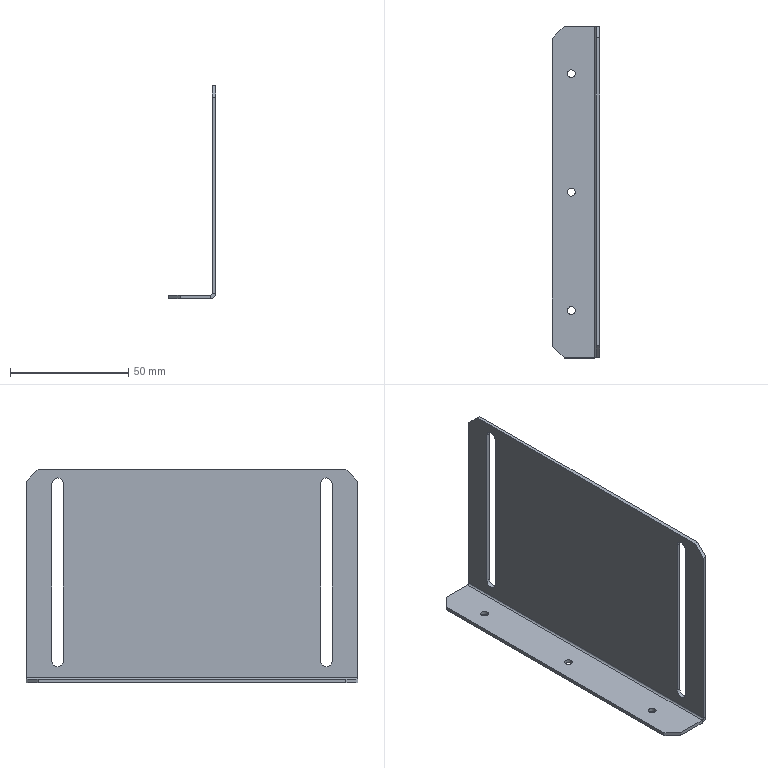Part | SolidWorks | features HoleWzd 2, BreakCorner 1, FlatPattern 1, SMBaseFlange 1, SheetMetal 1 | 1 solid | 34 faces | box 20 x 140 x 90 mm | volume 21403 mm3 | plane 20 | cylinder 14 | commonest cylinder face diameters 3.3 x6 4.8 x6 1.473 x1 4.473 x1
STEP:
#1=CARTESIAN_POINT('',(20.,56.75,86.4));
#2=VERTEX_POINT('',#1);
#3=CARTESIAN_POINT('',(20.,59.15,84.));
#4=VERTEX_POINT('',#3);
#5=CARTESIAN_POINT('',(20.,56.75,84.));
#6=DIRECTION('',(-1.,0.,0.));
#7=DIRECTION('',(0.,0.,1.));
#8=AXIS2_PLACEMENT_3D('',#5,#6,#7);
#9=CIRCLE('',#8,2.4);
#10=EDGE_CURVE('',#2,#4,#9,.T.);
#11=ORIENTED_EDGE('',*,*,#10,.F.);
#12=CARTESIAN_POINT('',(18.5,56.75,86.4));
#13=VERTEX_POINT('',#12);
#14=CARTESIAN_POINT('',(18.5,56.75,86.4));
#15=DIRECTION('',(-1.,0.,0.));
#16=VECTOR('',#15,1000.);
#17=LINE('',#14,#16);
#18=EDGE_CURVE('',#2,#13,#17,.T.);
#19=ORIENTED_EDGE('',*,*,#18,.T.);
#20=CARTESIAN_POINT('',(18.5,59.15,84.));
#21=VERTEX_POINT('',#20);
#22=CARTESIAN_POINT('',(18.5,56.75,84.));
#23=DIRECTION('',(-1.,0.,0.));
#24=DIRECTION('',(0.,0.,1.));
#25=AXIS2_PLACEMENT_3D('',#22,#23,#24);
#26=CIRCLE('',#25,2.4);
#27=EDGE_CURVE('',#13,#21,#26,.T.);
#28=ORIENTED_EDGE('',*,*,#27,.T.);
#29=CARTESIAN_POINT('',(20.,59.15,84.));
#30=DIRECTION('',(1.,0.,0.));
#31=VECTOR('',#30,1000.);
#32=LINE('',#29,#31);
#33=EDGE_CURVE('',#21,#4,#32,.T.);
#34=ORIENTED_EDGE('',*,*,#33,.T.);
#35=EDGE_LOOP('',(#11,#19,#28,#34));
#36=FACE_OUTER_BOUND('',#35,.T.);
#37=CARTESIAN_POINT('',(18.5,56.75,84.));
#38=DIRECTION('',(-1.,0.,0.));
#39=DIRECTION('',(0.,0.,1.));
#40=AXIS2_PLACEMENT_3D('',#37,#38,#39);
#41=CYLINDRICAL_SURFACE('',#40,2.4);
#42=ADVANCED_FACE('',(#36),#41,.F.);
#43=CARTESIAN_POINT('',(20.,-56.75,86.4));
#44=VERTEX_POINT('',#43);
#45=CARTESIAN_POINT('',(20.,-54.35,84.));
#46=VERTEX_POINT('',#45);
#47=CARTESIAN_POINT('',(20.,-56.75,84.));
#48=DIRECTION('',(-1.,0.,0.));
#49=DIRECTION('',(0.,0.,1.));
#50=AXIS2_PLACEMENT_3D('',#47,#48,#49);
#51=CIRCLE('',#50,2.4);
#52=EDGE_CURVE('',#44,#46,#51,.T.);
#53=ORIENTED_EDGE('',*,*,#52,.F.);
#54=CARTESIAN_POINT('',(18.5,-56.75,86.4));
#55=VERTEX_POINT('',#54);
#56=CARTESIAN_POINT('',(18.5,-56.75,86.4));
#57=DIRECTION('',(-1.,0.,0.));
#58=VECTOR('',#57,1000.);
#59=LINE('',#56,#58);
#60=EDGE_CURVE('',#44,#55,#59,.T.);
#61=ORIENTED_EDGE('',*,*,#60,.T.);
#62=CARTESIAN_POINT('',(18.5,-54.35,84.));
#63=VERTEX_POINT('',#62);
#64=CARTESIAN_POINT('',(18.5,-56.75,84.));
#65=DIRECTION('',(-1.,0.,0.));
#66=DIRECTION('',(0.,0.,1.));
#67=AXIS2_PLACEMENT_3D('',#64,#65,#66);
#68=CIRCLE('',#67,2.4);
#69=EDGE_CURVE('',#55,#63,#68,.T.);
#70=ORIENTED_EDGE('',*,*,#69,.T.);
#71=CARTESIAN_POINT('',(20.,-54.35,84.));
#72=DIRECTION('',(1.,0.,0.));
#73=VECTOR('',#72,1000.);
#74=LINE('',#71,#73);
#75=EDGE_CURVE('',#63,#46,#74,.T.);
#76=ORIENTED_EDGE('',*,*,#75,.T.);
#77=EDGE_LOOP('',(#53,#61,#70,#76));
#78=FACE_OUTER_BOUND('',#77,.T.);
#79=CARTESIAN_POINT('',(18.5,-56.75,84.));
#80=DIRECTION('',(-1.,0.,0.));
#81=DIRECTION('',(0.,0.,1.));
#82=AXIS2_PLACEMENT_3D('',#79,#80,#81);
#83=CYLINDRICAL_SURFACE('',#82,2.4);
#84=ADVANCED_FACE('',(#78),#83,.F.);
#85=CARTESIAN_POINT('',(6.35,50.,0.));
#86=VERTEX_POINT('',#85);
#87=CARTESIAN_POINT('',(9.65,50.,0.));
#88=VERTEX_POINT('',#87);
#89=CARTESIAN_POINT('',(8.,50.,0.));
#90=DIRECTION('',(0.,0.,1.));
#91=DIRECTION('',(1.,0.,0.));
#92=AXIS2_PLACEMENT_3D('',#89,#90,#91);
#93=CIRCLE('',#92,1.65);
#94=EDGE_CURVE('',#86,#88,#93,.T.);
#95=ORIENTED_EDGE('',*,*,#94,.F.);
#96=CARTESIAN_POINT('',(6.35,50.,1.5));
#97=VERTEX_POINT('',#96);
#98=CARTESIAN_POINT('',(6.35,50.,1.5));
#99=DIRECTION('',(0.,0.,1.));
#100=VECTOR('',#99,1000.);
#101=LINE('',#98,#100);
#102=EDGE_CURVE('',#86,#97,#101,.T.);
#103=ORIENTED_EDGE('',*,*,#102,.T.);
#104=CARTESIAN_POINT('',(9.65,50.,1.5));
#105=VERTEX_POINT('',#104);
#106=CARTESIAN_POINT('',(8.,50.,1.5));
#107=DIRECTION('',(0.,0.,1.));
#108=DIRECTION('',(1.,0.,0.));
#109=AXIS2_PLACEMENT_3D('',#106,#107,#108);
#110=CIRCLE('',#109,1.65);
#111=EDGE_CURVE('',#97,#105,#110,.T.);
#112=ORIENTED_EDGE('',*,*,#111,.T.);
#113=CARTESIAN_POINT('',(9.65,50.,1.5));
#114=DIRECTION('',(0.,0.,1.));
#115=VECTOR('',#114,1000.);
#116=LINE('',#113,#115);
#117=EDGE_CURVE('',#88,#105,#116,.T.);
#118=ORIENTED_EDGE('',*,*,#117,.F.);
#119=EDGE_LOOP('',(#95,#103,#112,#118));
#120=FACE_OUTER_BOUND('',#119,.T.);
#121=CARTESIAN_POINT('',(8.,50.,1.5));
#122=DIRECTION('',(0.,0.,1.));
#123=DIRECTION('',(1.,0.,0.));
#124=AXIS2_PLACEMENT_3D('',#121,#122,#123);
#125=CYLINDRICAL_SURFACE('',#124,1.65);
#126=ADVANCED_FACE('',(#120),#125,.F.);
#127=CARTESIAN_POINT('',(6.35,-50.,0.));
#128=VERTEX_POINT('',#127);
#129=CARTESIAN_POINT('',(9.65,-50.,0.));
#130=VERTEX_POINT('',#129);
#131=CARTESIAN_POINT('',(8.,-50.,0.));
#132=DIRECTION('',(0.,0.,1.));
#133=DIRECTION('',(1.,0.,0.));
#134=AXIS2_PLACEMENT_3D('',#131,#132,#133);
#135=CIRCLE('',#134,1.65);
#136=EDGE_CURVE('',#128,#130,#135,.T.);
#137=ORIENTED_EDGE('',*,*,#136,.F.);
#138=CARTESIAN_POINT('',(6.35,-50.,1.5));
#139=VERTEX_POINT('',#138);
#140=CARTESIAN_POINT('',(6.35,-50.,1.5));
#141=DIRECTION('',(0.,0.,1.));
#142=VECTOR('',#141,1000.);
#143=LINE('',#140,#142);
#144=EDGE_CURVE('',#128,#139,#143,.T.);
#145=ORIENTED_EDGE('',*,*,#144,.T.);
#146=CARTESIAN_POINT('',(9.65,-50.,1.5));
#147=VERTEX_POINT('',#146);
#148=CARTESIAN_POINT('',(8.,-50.,1.5));
#149=DIRECTION('',(0.,0.,1.));
#150=DIRECTION('',(1.,0.,0.));
#151=AXIS2_PLACEMENT_3D('',#148,#149,#150);
#152=CIRCLE('',#151,1.65);
#153=EDGE_CURVE('',#139,#147,#152,.T.);
#154=ORIENTED_EDGE('',*,*,#153,.T.);
#155=CARTESIAN_POINT('',(9.65,-50.,1.5));
#156=DIRECTION('',(0.,0.,1.));
#157=VECTOR('',#156,1000.);
#158=LINE('',#155,#157);
#159=EDGE_CURVE('',#130,#147,#158,.T.);
#160=ORIENTED_EDGE('',*,*,#159,.F.);
#161=EDGE_LOOP('',(#137,#145,#154,#160));
#162=FACE_OUTER_BOUND('',#161,.T.);
#163=CARTESIAN_POINT('',(8.,-50.,1.5));
#164=DIRECTION('',(0.,0.,1.));
#165=DIRECTION('',(1.,0.,0.));
#166=AXIS2_PLACEMENT_3D('',#163,#164,#165);
#167=CYLINDRICAL_SURFACE('',#166,1.65);
#168=ADVANCED_FACE('',(#162),#167,.F.);
#169=CARTESIAN_POINT('',(6.35,0.,0.));
#170=VERTEX_POINT('',#169);
#171=CARTESIAN_POINT('',(9.65,0.,0.));
#172=VERTEX_POINT('',#171);
#173=CARTESIAN_POINT('',(8.,0.,0.));
#174=DIRECTION('',(0.,0.,1.));
#175=DIRECTION('',(1.,0.,0.));
#176=AXIS2_PLACEMENT_3D('',#173,#174,#175);
#177=CIRCLE('',#176,1.65);
#178=EDGE_CURVE('',#170,#172,#177,.T.);
#179=ORIENTED_EDGE('',*,*,#178,.F.);
#180=CARTESIAN_POINT('',(6.35,0.,1.5));
#181=VERTEX_POINT('',#180);
#182=CARTESIAN_POINT('',(6.35,0.,1.5));
#183=DIRECTION('',(0.,0.,1.));
#184=VECTOR('',#183,1000.);
#185=LINE('',#182,#184);
#186=EDGE_CURVE('',#170,#181,#185,.T.);
#187=ORIENTED_EDGE('',*,*,#186,.T.);
#188=CARTESIAN_POINT('',(9.65,0.,1.5));
#189=VERTEX_POINT('',#188);
#190=CARTESIAN_POINT('',(8.,0.,1.5));
#191=DIRECTION('',(0.,0.,1.));
#192=DIRECTION('',(1.,0.,0.));
#193=AXIS2_PLACEMENT_3D('',#190,#191,#192);
#194=CIRCLE('',#193,1.65);
#195=EDGE_CURVE('',#181,#189,#194,.T.);
#196=ORIENTED_EDGE('',*,*,#195,.T.);
#197=CARTESIAN_POINT('',(9.65,0.,1.5));
#198=DIRECTION('',(0.,0.,1.));
#199=VECTOR('',#198,1000.);
#200=LINE('',#197,#199);
#201=EDGE_CURVE('',#172,#189,#200,.T.);
#202=ORIENTED_EDGE('',*,*,#201,.F.);
#203=EDGE_LOOP('',(#179,#187,#196,#202));
#204=FACE_OUTER_BOUND('',#203,.T.);
#205=CARTESIAN_POINT('',(8.,0.,1.5));
#206=DIRECTION('',(0.,0.,1.));
#207=DIRECTION('',(1.,0.,0.));
#208=AXIS2_PLACEMENT_3D('',#205,#206,#207);
#209=CYLINDRICAL_SURFACE('',#208,1.65);
#210=ADVANCED_FACE('',(#204),#209,.F.);
#211=CARTESIAN_POINT('',(20.,59.15,9.));
#212=VERTEX_POINT('',#211);
#213=CARTESIAN_POINT('',(20.,59.15,9.));
#214=DIRECTION('',(0.,0.,1.));
#215=VECTOR('',#214,1000.);
#216=LINE('',#213,#215);
#217=EDGE_CURVE('',#212,#4,#216,.T.);
#218=ORIENTED_EDGE('',*,*,#217,.F.);
#219=CARTESIAN_POINT('',(20.,54.35,9.));
#220=VERTEX_POINT('',#219);
#221=CARTESIAN_POINT('',(20.,56.75,9.));
#222=DIRECTION('',(-1.,0.,0.));
#223=DIRECTION('',(0.,0.,1.));
#224=AXIS2_PLACEMENT_3D('',#221,#222,#223);
#225=CIRCLE('',#224,2.4);
#226=EDGE_CURVE('',#212,#220,#225,.T.);
#227=ORIENTED_EDGE('',*,*,#226,.T.);
#228=CARTESIAN_POINT('',(20.,54.35,84.));
#229=VERTEX_POINT('',#228);
#230=CARTESIAN_POINT('',(20.,54.35,9.));
#231=DIRECTION('',(0.,0.,1.));
#232=VECTOR('',#231,1000.);
#233=LINE('',#230,#232);
#234=EDGE_CURVE('',#220,#229,#233,.T.);
#235=ORIENTED_EDGE('',*,*,#234,.T.);
#236=CARTESIAN_POINT('',(20.,56.75,84.));
#237=DIRECTION('',(-1.,0.,0.));
#238=DIRECTION('',(0.,0.,1.));
#239=AXIS2_PLACEMENT_3D('',#236,#237,#238);
#240=CIRCLE('',#239,2.4);
#241=EDGE_CURVE('',#229,#2,#240,.T.);
#242=ORIENTED_EDGE('',*,*,#241,.T.);
#243=ORIENTED_EDGE('',*,*,#10,.T.);
#244=EDGE_LOOP('',(#218,#227,#235,#242,#243));
#245=FACE_BOUND('',#244,.T.);
#246=CARTESIAN_POINT('',(20.,70.,2.237));
#247=VERTEX_POINT('',#246);
#248=CARTESIAN_POINT('',(20.,70.,85.));
#249=VERTEX_POINT('',#248);
#250=CARTESIAN_POINT('',(20.,70.,0.));
#251=DIRECTION('',(0.,0.,1.));
#252=VECTOR('',#251,1000.);
#253=LINE('',#250,#252);
#254=EDGE_CURVE('',#247,#249,#253,.T.);
#255=ORIENTED_EDGE('',*,*,#254,.T.);
#256=CARTESIAN_POINT('',(20.,65.,90.));
#257=VERTEX_POINT('',#256);
#258=CARTESIAN_POINT('',(20.,112.5,42.5));
#259=DIRECTION('',(0.,-0.7071,0.7071));
#260=VECTOR('',#259,1000.);
#261=LINE('',#258,#260);
#262=EDGE_CURVE('',#249,#257,#261,.T.);
#263=ORIENTED_EDGE('',*,*,#262,.T.);
#264=CARTESIAN_POINT('',(20.,-65.,90.));
#265=VERTEX_POINT('',#264);
#266=CARTESIAN_POINT('',(20.,70.,90.));
#267=DIRECTION('',(0.,-1.,0.));
#268=VECTOR('',#267,1000.);
#269=LINE('',#266,#268);
#270=EDGE_CURVE('',#257,#265,#269,.T.);
#271=ORIENTED_EDGE('',*,*,#270,.T.);
#272=CARTESIAN_POINT('',(20.,-70.,85.));
#273=VERTEX_POINT('',#272);
#274=CARTESIAN_POINT('',(20.,-42.5,112.5));
#275=DIRECTION('',(0.,-0.7071,-0.7071));
#276=VECTOR('',#275,1000.);
#277=LINE('',#274,#276);
#278=EDGE_CURVE('',#265,#273,#277,.T.);
#279=ORIENTED_EDGE('',*,*,#278,.T.);
#280=CARTESIAN_POINT('',(20.,-70.,2.237));
#281=VERTEX_POINT('',#280);
#282=CARTESIAN_POINT('',(20.,-70.,0.));
#283=DIRECTION('',(0.,0.,1.));
#284=VECTOR('',#283,1000.);
#285=LINE('',#282,#284);
#286=EDGE_CURVE('',#281,#273,#285,.T.);
#287=ORIENTED_EDGE('',*,*,#286,.F.);
#288=CARTESIAN_POINT('',(20.,70.,2.237));
#289=DIRECTION('',(0.,-1.,0.));
#290=VECTOR('',#289,1000.);
#291=LINE('',#288,#290);
#292=EDGE_CURVE('',#247,#281,#291,.T.);
#293=ORIENTED_EDGE('',*,*,#292,.F.);
#294=EDGE_LOOP('',(#255,#263,#271,#279,#287,#293));
#295=FACE_OUTER_BOUND('',#294,.T.);
#296=CARTESIAN_POINT('',(20.,-59.15,9.));
#297=VERTEX_POINT('',#296);
#298=CARTESIAN_POINT('',(20.,-59.15,84.));
#299=VERTEX_POINT('',#298);
#300=CARTESIAN_POINT('',(20.,-59.15,9.));
#301=DIRECTION('',(0.,0.,1.));
#302=VECTOR('',#301,1000.);
#303=LINE('',#300,#302);
#304=EDGE_CURVE('',#297,#299,#303,.T.);
#305=ORIENTED_EDGE('',*,*,#304,.T.);
#306=CARTESIAN_POINT('',(20.,-56.75,84.));
#307=DIRECTION('',(-1.,0.,0.));
#308=DIRECTION('',(0.,0.,1.));
#309=AXIS2_PLACEMENT_3D('',#306,#307,#308);
#310=CIRCLE('',#309,2.4);
#311=EDGE_CURVE('',#299,#44,#310,.T.);
#312=ORIENTED_EDGE('',*,*,#311,.T.);
#313=ORIENTED_EDGE('',*,*,#52,.T.);
#314=CARTESIAN_POINT('',(20.,-54.35,9.));
#315=VERTEX_POINT('',#314);
#316=CARTESIAN_POINT('',(20.,-54.35,9.));
#317=DIRECTION('',(0.,0.,1.));
#318=VECTOR('',#317,1000.);
#319=LINE('',#316,#318);
#320=EDGE_CURVE('',#315,#46,#319,.T.);
#321=ORIENTED_EDGE('',*,*,#320,.F.);
#322=CARTESIAN_POINT('',(20.,-56.75,9.));
#323=DIRECTION('',(-1.,0.,0.));
#324=DIRECTION('',(0.,0.,1.));
#325=AXIS2_PLACEMENT_3D('',#322,#323,#324);
#326=CIRCLE('',#325,2.4);
#327=EDGE_CURVE('',#315,#297,#326,.T.);
#328=ORIENTED_EDGE('',*,*,#327,.T.);
#329=EDGE_LOOP('',(#305,#312,#313,#321,#328));
#330=FACE_BOUND('',#329,.T.);
#331=CARTESIAN_POINT('',(20.,70.,0.));
#332=DIRECTION('',(1.,0.,0.));
#333=DIRECTION('',(0.,0.,-1.));
#334=AXIS2_PLACEMENT_3D('',#331,#332,#333);
#335=PLANE('',#334);
#336=ADVANCED_FACE('',(#245,#295,#330),#335,.T.);
#337=CARTESIAN_POINT('',(8.,-50.,1.5));
#338=DIRECTION('',(0.,0.,1.));
#339=DIRECTION('',(1.,0.,0.));
#340=AXIS2_PLACEMENT_3D('',#337,#338,#339);
#341=CIRCLE('',#340,1.65);
#342=EDGE_CURVE('',#147,#139,#341,.T.);
#343=ORIENTED_EDGE('',*,*,#342,.F.);
#344=ORIENTED_EDGE('',*,*,#153,.F.);
#345=EDGE_LOOP('',(#343,#344));
#346=FACE_BOUND('',#345,.T.);
#347=CARTESIAN_POINT('',(8.,0.,1.5));
#348=DIRECTION('',(0.,0.,1.));
#349=DIRECTION('',(1.,0.,0.));
#350=AXIS2_PLACEMENT_3D('',#347,#348,#349);
#351=CIRCLE('',#350,1.65);
#352=EDGE_CURVE('',#189,#181,#351,.T.);
#353=ORIENTED_EDGE('',*,*,#352,.F.);
#354=ORIENTED_EDGE('',*,*,#195,.F.);
#355=EDGE_LOOP('',(#353,#354));
#356=FACE_BOUND('',#355,.T.);
#357=CARTESIAN_POINT('',(5.,70.,1.5));
#358=VERTEX_POINT('',#357);
#359=CARTESIAN_POINT('',(17.763,70.,1.5));
#360=VERTEX_POINT('',#359);
#361=CARTESIAN_POINT('',(0.,70.,1.5));
#362=DIRECTION('',(1.,0.,0.));
#363=VECTOR('',#362,1000.);
#364=LINE('',#361,#363);
#365=EDGE_CURVE('',#358,#360,#364,.T.);
#366=ORIENTED_EDGE('',*,*,#365,.F.);
#367=CARTESIAN_POINT('',(0.,65.,1.5));
#368=VERTEX_POINT('',#367);
#369=CARTESIAN_POINT('',(0.,65.,1.5));
#370=DIRECTION('',(-0.7071,-0.7071,0.));
#371=VECTOR('',#370,1000.);
#372=LINE('',#369,#371);
#373=EDGE_CURVE('',#358,#368,#372,.T.);
#374=ORIENTED_EDGE('',*,*,#373,.T.);
#375=CARTESIAN_POINT('',(0.,-65.,1.5));
#376=VERTEX_POINT('',#375);
#377=CARTESIAN_POINT('',(0.,70.,1.5));
#378=DIRECTION('',(0.,-1.,0.));
#379=VECTOR('',#378,1000.);
#380=LINE('',#377,#379);
#381=EDGE_CURVE('',#368,#376,#380,.T.);
#382=ORIENTED_EDGE('',*,*,#381,.T.);
#383=CARTESIAN_POINT('',(5.,-70.,1.5));
#384=VERTEX_POINT('',#383);
#385=CARTESIAN_POINT('',(5.,-70.,1.5));
#386=DIRECTION('',(0.7071,-0.7071,0.));
#387=VECTOR('',#386,1000.);
#388=LINE('',#385,#387);
#389=EDGE_CURVE('',#376,#384,#388,.T.);
#390=ORIENTED_EDGE('',*,*,#389,.T.);
#391=CARTESIAN_POINT('',(17.763,-70.,1.5));
#392=VERTEX_POINT('',#391);
#393=CARTESIAN_POINT('',(0.,-70.,1.5));
#394=DIRECTION('',(1.,0.,0.));
#395=VECTOR('',#394,1000.);
#396=LINE('',#393,#395);
#397=EDGE_CURVE('',#384,#392,#396,.T.);
#398=ORIENTED_EDGE('',*,*,#397,.T.);
#399=CARTESIAN_POINT('',(17.763,70.,1.5));
#400=DIRECTION('',(0.,-1.,0.));
#401=VECTOR('',#400,1000.);
#402=LINE('',#399,#401);
#403=EDGE_CURVE('',#360,#392,#402,.T.);
#404=ORIENTED_EDGE('',*,*,#403,.F.);
#405=EDGE_LOOP('',(#366,#374,#382,#390,#398,#404));
#406=FACE_OUTER_BOUND('',#405,.T.);
#407=CARTESIAN_POINT('',(8.,50.,1.5));
#408=DIRECTION('',(0.,0.,1.));
#409=DIRECTION('',(1.,0.,0.));
#410=AXIS2_PLACEMENT_3D('',#407,#408,#409);
#411=CIRCLE('',#410,1.65);
#412=EDGE_CURVE('',#105,#97,#411,.T.);
#413=ORIENTED_EDGE('',*,*,#412,.F.);
#414=ORIENTED_EDGE('',*,*,#111,.F.);
#415=EDGE_LOOP('',(#413,#414));
#416=FACE_BOUND('',#415,.T.);
#417=CARTESIAN_POINT('',(0.,70.,1.5));
#418=DIRECTION('',(0.,0.,-1.));
#419=DIRECTION('',(-1.,0.,0.));
#420=AXIS2_PLACEMENT_3D('',#417,#418,#419);
#421=PLANE('',#420);
#422=ADVANCED_FACE('',(#346,#356,#406,#416),#421,.F.);
#423=CARTESIAN_POINT('',(18.5,70.,2.237));
#424=VERTEX_POINT('',#423);
#425=CARTESIAN_POINT('',(20.,70.,2.237));
#426=DIRECTION('',(-1.,0.,0.));
#427=VECTOR('',#426,1000.);
#428=LINE('',#425,#427);
#429=EDGE_CURVE('',#247,#424,#428,.T.);
#430=ORIENTED_EDGE('',*,*,#429,.F.);
#431=CARTESIAN_POINT('',(17.763,70.,0.));
#432=VERTEX_POINT('',#431);
#433=CARTESIAN_POINT('',(17.763,70.,2.237));
#434=DIRECTION('',(0.,-1.,0.));
#435=DIRECTION('',(0.,0.,1.));
#436=AXIS2_PLACEMENT_3D('',#433,#434,#435);
#437=CIRCLE('',#436,2.237);
#438=EDGE_CURVE('',#432,#247,#437,.T.);
#439=ORIENTED_EDGE('',*,*,#438,.F.);
#440=CARTESIAN_POINT('',(17.763,70.,1.5));
#441=DIRECTION('',(0.,0.,-1.));
#442=VECTOR('',#441,1000.);
#443=LINE('',#440,#442);
#444=EDGE_CURVE('',#360,#432,#443,.T.);
#445=ORIENTED_EDGE('',*,*,#444,.F.);
#446=CARTESIAN_POINT('',(17.763,70.,2.237));
#447=DIRECTION('',(0.,-1.,0.));
#448=DIRECTION('',(1.,0.,0.));
#449=AXIS2_PLACEMENT_3D('',#446,#447,#448);
#450=CIRCLE('',#449,0.7366);
#451=EDGE_CURVE('',#360,#424,#450,.T.);
#452=ORIENTED_EDGE('',*,*,#451,.T.);
#453=EDGE_LOOP('',(#430,#439,#445,#452));
#454=FACE_OUTER_BOUND('',#453,.T.);
#455=CARTESIAN_POINT('',(20.,70.,2.237));
#456=DIRECTION('',(0.,1.,0.));
#457=DIRECTION('',(0.,0.,1.));
#458=AXIS2_PLACEMENT_3D('',#455,#456,#457);
#459=PLANE('',#458);
#460=ADVANCED_FACE('',(#454),#459,.T.);
#461=CARTESIAN_POINT('',(18.5,70.,85.));
#462=VERTEX_POINT('',#461);
#463=CARTESIAN_POINT('',(18.5,70.,0.));
#464=DIRECTION('',(0.,0.,1.));
#465=VECTOR('',#464,1000.);
#466=LINE('',#463,#465);
#467=EDGE_CURVE('',#424,#462,#466,.T.);
#468=ORIENTED_EDGE('',*,*,#467,.T.);
#469=CARTESIAN_POINT('',(17.763,70.,85.));
#470=DIRECTION('',(1.,0.,0.));
#471=VECTOR('',#470,1000.);
#472=LINE('',#469,#471);
#473=EDGE_CURVE('',#462,#249,#472,.T.);
#474=ORIENTED_EDGE('',*,*,#473,.T.);
#475=ORIENTED_EDGE('',*,*,#254,.F.);
#476=ORIENTED_EDGE('',*,*,#429,.T.);
#477=EDGE_LOOP('',(#468,#474,#475,#476));
#478=FACE_OUTER_BOUND('',#477,.T.);
#479=CARTESIAN_POINT('',(17.763,70.,1.5));
#480=DIRECTION('',(0.,1.,0.));
#481=DIRECTION('',(0.,0.,1.));
#482=AXIS2_PLACEMENT_3D('',#479,#480,#481);
#483=PLANE('',#482);
#484=ADVANCED_FACE('',(#478),#483,.T.);
#485=CARTESIAN_POINT('',(17.763,-70.,0.));
#486=VERTEX_POINT('',#485);
#487=CARTESIAN_POINT('',(17.763,-70.,0.));
#488=DIRECTION('',(0.,0.,1.));
#489=VECTOR('',#488,1000.);
#490=LINE('',#487,#489);
#491=EDGE_CURVE('',#486,#392,#490,.T.);
#492=ORIENTED_EDGE('',*,*,#491,.F.);
#493=CARTESIAN_POINT('',(17.763,-70.,2.237));
#494=DIRECTION('',(0.,-1.,0.));
#495=DIRECTION('',(0.,0.,1.));
#496=AXIS2_PLACEMENT_3D('',#493,#494,#495);
#497=CIRCLE('',#496,2.237);
#498=EDGE_CURVE('',#486,#281,#497,.T.);
#499=ORIENTED_EDGE('',*,*,#498,.T.);
#500=CARTESIAN_POINT('',(18.5,-70.,2.237));
#501=VERTEX_POINT('',#500);
#502=CARTESIAN_POINT('',(18.5,-70.,2.237));
#503=DIRECTION('',(1.,0.,0.));
#504=VECTOR('',#503,1000.);
#505=LINE('',#502,#504);
#506=EDGE_CURVE('',#501,#281,#505,.T.);
#507=ORIENTED_EDGE('',*,*,#506,.F.);
#508=CARTESIAN_POINT('',(17.763,-70.,2.237));
#509=DIRECTION('',(0.,-1.,0.));
#510=DIRECTION('',(1.,0.,0.));
#511=AXIS2_PLACEMENT_3D('',#508,#509,#510);
#512=CIRCLE('',#511,0.7366);
#513=EDGE_CURVE('',#392,#501,#512,.T.);
#514=ORIENTED_EDGE('',*,*,#513,.F.);
#515=EDGE_LOOP('',(#492,#499,#507,#514));
#516=FACE_OUTER_BOUND('',#515,.T.);
#517=CARTESIAN_POINT('',(17.763,-70.,0.));
#518=DIRECTION('',(0.,-1.,0.));
#519=DIRECTION('',(0.,0.,-1.));
#520=AXIS2_PLACEMENT_3D('',#517,#518,#519);
#521=PLANE('',#520);
#522=ADVANCED_FACE('',(#516),#521,.T.);
#523=ORIENTED_EDGE('',*,*,#397,.F.);
#524=CARTESIAN_POINT('',(5.,-70.,0.));
#525=VERTEX_POINT('',#524);
#526=CARTESIAN_POINT('',(5.,-70.,2.237));
#527=DIRECTION('',(0.,0.,-1.));
#528=VECTOR('',#527,1000.);
#529=LINE('',#526,#528);
#530=EDGE_CURVE('',#384,#525,#529,.T.);
#531=ORIENTED_EDGE('',*,*,#530,.T.);
#532=CARTESIAN_POINT('',(0.,-70.,0.));
#533=DIRECTION('',(1.,0.,0.));
#534=VECTOR('',#533,1000.);
#535=LINE('',#532,#534);
#536=EDGE_CURVE('',#525,#486,#535,.T.);
#537=ORIENTED_EDGE('',*,*,#536,.T.);
#538=ORIENTED_EDGE('',*,*,#491,.T.);
#539=EDGE_LOOP('',(#523,#531,#537,#538));
#540=FACE_OUTER_BOUND('',#539,.T.);
#541=CARTESIAN_POINT('',(18.5,-70.,2.237));
#542=DIRECTION('',(0.,-1.,0.));
#543=DIRECTION('',(0.,0.,-1.));
#544=AXIS2_PLACEMENT_3D('',#541,#542,#543);
#545=PLANE('',#544);
#546=ADVANCED_FACE('',(#540),#545,.T.);
#547=CARTESIAN_POINT('',(18.5,59.15,9.));
#548=VERTEX_POINT('',#547);
#549=CARTESIAN_POINT('',(18.5,59.15,9.));
#550=DIRECTION('',(0.,0.,1.));
#551=VECTOR('',#550,1000.);
#552=LINE('',#549,#551);
#553=EDGE_CURVE('',#548,#21,#552,.T.);
#554=ORIENTED_EDGE('',*,*,#553,.T.);
#555=ORIENTED_EDGE('',*,*,#27,.F.);
#556=CARTESIAN_POINT('',(18.5,54.35,84.));
#557=VERTEX_POINT('',#556);
#558=CARTESIAN_POINT('',(18.5,56.75,84.));
#559=DIRECTION('',(-1.,0.,0.));
#560=DIRECTION('',(0.,0.,1.));
#561=AXIS2_PLACEMENT_3D('',#558,#559,#560);
#562=CIRCLE('',#561,2.4);
#563=EDGE_CURVE('',#557,#13,#562,.T.);
#564=ORIENTED_EDGE('',*,*,#563,.F.);
#565=CARTESIAN_POINT('',(18.5,54.35,9.));
#566=VERTEX_POINT('',#565);
#567=CARTESIAN_POINT('',(18.5,54.35,9.));
#568=DIRECTION('',(0.,0.,1.));
#569=VECTOR('',#568,1000.);
#570=LINE('',#567,#569);
#571=EDGE_CURVE('',#566,#557,#570,.T.);
#572=ORIENTED_EDGE('',*,*,#571,.F.);
#573=CARTESIAN_POINT('',(18.5,56.75,9.));
#574=DIRECTION('',(-1.,0.,0.));
#575=DIRECTION('',(0.,0.,1.));
#576=AXIS2_PLACEMENT_3D('',#573,#574,#575);
#577=CIRCLE('',#576,2.4);
#578=EDGE_CURVE('',#548,#566,#577,.T.);
#579=ORIENTED_EDGE('',*,*,#578,.F.);
#580=EDGE_LOOP('',(#554,#555,#564,#572,#579));
#581=FACE_BOUND('',#580,.T.);
#582=CARTESIAN_POINT('',(18.5,-54.35,9.));
#583=VERTEX_POINT('',#582);
#584=CARTESIAN_POINT('',(18.5,-54.35,9.));
#585=DIRECTION('',(0.,0.,1.));
#586=VECTOR('',#585,1000.);
#587=LINE('',#584,#586);
#588=EDGE_CURVE('',#583,#63,#587,.T.);
#589=ORIENTED_EDGE('',*,*,#588,.T.);
#590=ORIENTED_EDGE('',*,*,#69,.F.);
#591=CARTESIAN_POINT('',(18.5,-59.15,84.));
#592=VERTEX_POINT('',#591);
#593=CARTESIAN_POINT('',(18.5,-56.75,84.));
#594=DIRECTION('',(-1.,0.,0.));
#595=DIRECTION('',(0.,0.,1.));
#596=AXIS2_PLACEMENT_3D('',#593,#594,#595);
#597=CIRCLE('',#596,2.4);
#598=EDGE_CURVE('',#592,#55,#597,.T.);
#599=ORIENTED_EDGE('',*,*,#598,.F.);
#600=CARTESIAN_POINT('',(18.5,-59.15,9.));
#601=VERTEX_POINT('',#600);
#602=CARTESIAN_POINT('',(18.5,-59.15,9.));
#603=DIRECTION('',(0.,0.,1.));
#604=VECTOR('',#603,1000.);
#605=LINE('',#602,#604);
#606=EDGE_CURVE('',#601,#592,#605,.T.);
#607=ORIENTED_EDGE('',*,*,#606,.F.);
#608=CARTESIAN_POINT('',(18.5,-56.75,9.));
#609=DIRECTION('',(-1.,0.,0.));
#610=DIRECTION('',(0.,0.,1.));
#611=AXIS2_PLACEMENT_3D('',#608,#609,#610);
#612=CIRCLE('',#611,2.4);
#613=EDGE_CURVE('',#583,#601,#612,.T.);
#614=ORIENTED_EDGE('',*,*,#613,.F.);
#615=EDGE_LOOP('',(#589,#590,#599,#607,#614));
#616=FACE_BOUND('',#615,.T.);
#617=CARTESIAN_POINT('',(18.5,65.,90.));
#618=VERTEX_POINT('',#617);
#619=CARTESIAN_POINT('',(18.5,-65.,90.));
#620=VERTEX_POINT('',#619);
#621=CARTESIAN_POINT('',(18.5,70.,90.));
#622=DIRECTION('',(0.,-1.,0.));
#623=VECTOR('',#622,1000.);
#624=LINE('',#621,#623);
#625=EDGE_CURVE('',#618,#620,#624,.T.);
#626=ORIENTED_EDGE('',*,*,#625,.F.);
#627=CARTESIAN_POINT('',(18.5,65.,90.));
#628=DIRECTION('',(0.,0.7071,-0.7071));
#629=VECTOR('',#628,1000.);
#630=LINE('',#627,#629);
#631=EDGE_CURVE('',#618,#462,#630,.T.);
#632=ORIENTED_EDGE('',*,*,#631,.T.);
#633=ORIENTED_EDGE('',*,*,#467,.F.);
#634=CARTESIAN_POINT('',(18.5,70.,2.237));
#635=DIRECTION('',(0.,-1.,0.));
#636=VECTOR('',#635,1000.);
#637=LINE('',#634,#636);
#638=EDGE_CURVE('',#424,#501,#637,.T.);
#639=ORIENTED_EDGE('',*,*,#638,.T.);
#640=CARTESIAN_POINT('',(18.5,-70.,85.));
#641=VERTEX_POINT('',#640);
#642=CARTESIAN_POINT('',(18.5,-70.,0.));
#643=DIRECTION('',(0.,0.,1.));
#644=VECTOR('',#643,1000.);
#645=LINE('',#642,#644);
#646=EDGE_CURVE('',#501,#641,#645,.T.);
#647=ORIENTED_EDGE('',*,*,#646,.T.);
#648=CARTESIAN_POINT('',(18.5,-70.,85.));
#649=DIRECTION('',(0.,0.7071,0.7071));
#650=VECTOR('',#649,1000.);
#651=LINE('',#648,#650);
#652=EDGE_CURVE('',#641,#620,#651,.T.);
#653=ORIENTED_EDGE('',*,*,#652,.T.);
#654=EDGE_LOOP('',(#626,#632,#633,#639,#647,#653));
#655=FACE_OUTER_BOUND('',#654,.T.);
#656=CARTESIAN_POINT('',(18.5,70.,0.));
#657=DIRECTION('',(1.,0.,0.));
#658=DIRECTION('',(0.,0.,-1.));
#659=AXIS2_PLACEMENT_3D('',#656,#657,#658);
#660=PLANE('',#659);
#661=ADVANCED_FACE('',(#581,#616,#655),#660,.F.);
#662=ORIENTED_EDGE('',*,*,#270,.F.);
#663=CARTESIAN_POINT('',(20.,65.,90.));
#664=DIRECTION('',(-1.,0.,0.));
#665=VECTOR('',#664,1000.);
#666=LINE('',#663,#665);
#667=EDGE_CURVE('',#257,#618,#666,.T.);
#668=ORIENTED_EDGE('',*,*,#667,.T.);
#669=ORIENTED_EDGE('',*,*,#625,.T.);
#670=CARTESIAN_POINT('',(20.,-65.,90.));
#671=DIRECTION('',(1.,0.,0.));
#672=VECTOR('',#671,1000.);
#673=LINE('',#670,#672);
#674=EDGE_CURVE('',#620,#265,#673,.T.);
#675=ORIENTED_EDGE('',*,*,#674,.T.);
#676=EDGE_LOOP('',(#662,#668,#669,#675));
#677=FACE_OUTER_BOUND('',#676,.T.);
#678=CARTESIAN_POINT('',(20.,70.,90.));
#679=DIRECTION('',(0.,0.,1.));
#680=DIRECTION('',(1.,0.,0.));
#681=AXIS2_PLACEMENT_3D('',#678,#679,#680);
#682=PLANE('',#681);
#683=ADVANCED_FACE('',(#677),#682,.T.);
#684=ORIENTED_EDGE('',*,*,#498,.F.);
#685=CARTESIAN_POINT('',(17.763,70.,0.));
#686=DIRECTION('',(0.,-1.,0.));
#687=VECTOR('',#686,1000.);
#688=LINE('',#685,#687);
#689=EDGE_CURVE('',#432,#486,#688,.T.);
#690=ORIENTED_EDGE('',*,*,#689,.F.);
#691=ORIENTED_EDGE('',*,*,#438,.T.);
#692=ORIENTED_EDGE('',*,*,#292,.T.);
#693=EDGE_LOOP('',(#684,#690,#691,#692));
#694=FACE_OUTER_BOUND('',#693,.T.);
#695=CARTESIAN_POINT('',(17.763,70.,2.237));
#696=DIRECTION('',(0.,-1.,0.));
#697=DIRECTION('',(0.,0.,-1.));
#698=AXIS2_PLACEMENT_3D('',#695,#696,#697);
#699=CYLINDRICAL_SURFACE('',#698,2.237);
#700=ADVANCED_FACE('',(#694),#699,.T.);
#701=CARTESIAN_POINT('',(8.,50.,0.));
#702=DIRECTION('',(0.,0.,1.));
#703=DIRECTION('',(1.,0.,0.));
#704=AXIS2_PLACEMENT_3D('',#701,#702,#703);
#705=CIRCLE('',#704,1.65);
#706=EDGE_CURVE('',#88,#86,#705,.T.);
#707=ORIENTED_EDGE('',*,*,#706,.T.);
#708=ORIENTED_EDGE('',*,*,#94,.T.);
#709=EDGE_LOOP('',(#707,#708));
#710=FACE_BOUND('',#709,.T.);
#711=CARTESIAN_POINT('',(8.,-50.,0.));
#712=DIRECTION('',(0.,0.,1.));
#713=DIRECTION('',(1.,0.,0.));
#714=AXIS2_PLACEMENT_3D('',#711,#712,#713);
#715=CIRCLE('',#714,1.65);
#716=EDGE_CURVE('',#130,#128,#715,.T.);
#717=ORIENTED_EDGE('',*,*,#716,.T.);
#718=ORIENTED_EDGE('',*,*,#136,.T.);
#719=EDGE_LOOP('',(#717,#718));
#720=FACE_BOUND('',#719,.T.);
#721=CARTESIAN_POINT('',(8.,0.,0.));
#722=DIRECTION('',(0.,0.,1.));
#723=DIRECTION('',(1.,0.,0.));
#724=AXIS2_PLACEMENT_3D('',#721,#722,#723);
#725=CIRCLE('',#724,1.65);
#726=EDGE_CURVE('',#172,#170,#725,.T.);
#727=ORIENTED_EDGE('',*,*,#726,.T.);
#728=ORIENTED_EDGE('',*,*,#178,.T.);
#729=EDGE_LOOP('',(#727,#728));
#730=FACE_BOUND('',#729,.T.);
#731=CARTESIAN_POINT('',(0.,65.,0.));
#732=VERTEX_POINT('',#731);
#733=CARTESIAN_POINT('',(0.,-65.,0.));
#734=VERTEX_POINT('',#733);
#735=CARTESIAN_POINT('',(0.,70.,0.));
#736=DIRECTION('',(0.,-1.,0.));
#737=VECTOR('',#736,1000.);
#738=LINE('',#735,#737);
#739=EDGE_CURVE('',#732,#734,#738,.T.);
#740=ORIENTED_EDGE('',*,*,#739,.F.);
#741=CARTESIAN_POINT('',(5.,70.,0.));
#742=VERTEX_POINT('',#741);
#743=CARTESIAN_POINT('',(2.5,67.5,0.));
#744=DIRECTION('',(0.7071,0.7071,0.));
#745=VECTOR('',#744,1000.);
#746=LINE('',#743,#745);
#747=EDGE_CURVE('',#732,#742,#746,.T.);
#748=ORIENTED_EDGE('',*,*,#747,.T.);
#749=CARTESIAN_POINT('',(0.,70.,0.));
#750=DIRECTION('',(1.,0.,0.));
#751=VECTOR('',#750,1000.);
#752=LINE('',#749,#751);
#753=EDGE_CURVE('',#742,#432,#752,.T.);
#754=ORIENTED_EDGE('',*,*,#753,.T.);
#755=ORIENTED_EDGE('',*,*,#689,.T.);
#756=ORIENTED_EDGE('',*,*,#536,.F.);
#757=CARTESIAN_POINT('',(-67.5,2.5,0.));
#758=DIRECTION('',(-0.7071,0.7071,0.));
#759=VECTOR('',#758,1000.);
#760=LINE('',#757,#759);
#761=EDGE_CURVE('',#525,#734,#760,.T.);
#762=ORIENTED_EDGE('',*,*,#761,.T.);
#763=EDGE_LOOP('',(#740,#748,#754,#755,#756,#762));
#764=FACE_OUTER_BOUND('',#763,.T.);
#765=CARTESIAN_POINT('',(0.,70.,0.));
#766=DIRECTION('',(0.,0.,-1.));
#767=DIRECTION('',(-1.,0.,0.));
#768=AXIS2_PLACEMENT_3D('',#765,#766,#767);
#769=PLANE('',#768);
#770=ADVANCED_FACE('',(#710,#720,#730,#764),#769,.T.);
#771=ORIENTED_EDGE('',*,*,#381,.F.);
#772=CARTESIAN_POINT('',(0.,65.,1.5));
#773=DIRECTION('',(0.,0.,-1.));
#774=VECTOR('',#773,1000.);
#775=LINE('',#772,#774);
#776=EDGE_CURVE('',#368,#732,#775,.T.);
#777=ORIENTED_EDGE('',*,*,#776,.T.);
#778=ORIENTED_EDGE('',*,*,#739,.T.);
#779=CARTESIAN_POINT('',(0.,-65.,1.5));
#780=DIRECTION('',(0.,0.,1.));
#781=VECTOR('',#780,1000.);
#782=LINE('',#779,#781);
#783=EDGE_CURVE('',#734,#376,#782,.T.);
#784=ORIENTED_EDGE('',*,*,#783,.T.);
#785=EDGE_LOOP('',(#771,#777,#778,#784));
#786=FACE_OUTER_BOUND('',#785,.T.);
#787=CARTESIAN_POINT('',(0.,70.,1.5));
#788=DIRECTION('',(-1.,0.,0.));
#789=DIRECTION('',(0.,0.,1.));
#790=AXIS2_PLACEMENT_3D('',#787,#788,#789);
#791=PLANE('',#790);
#792=ADVANCED_FACE('',(#786),#791,.T.);
#793=ORIENTED_EDGE('',*,*,#513,.T.);
#794=ORIENTED_EDGE('',*,*,#638,.F.);
#795=ORIENTED_EDGE('',*,*,#451,.F.);
#796=ORIENTED_EDGE('',*,*,#403,.T.);
#797=EDGE_LOOP('',(#793,#794,#795,#796));
#798=FACE_OUTER_BOUND('',#797,.T.);
#799=CARTESIAN_POINT('',(17.763,70.,2.237));
#800=DIRECTION('',(0.,-1.,0.));
#801=DIRECTION('',(0.,0.,-1.));
#802=AXIS2_PLACEMENT_3D('',#799,#800,#801);
#803=CYLINDRICAL_SURFACE('',#802,0.7366);
#804=ADVANCED_FACE('',(#798),#803,.F.);
#805=ORIENTED_EDGE('',*,*,#753,.F.);
#806=CARTESIAN_POINT('',(5.,70.,2.237));
#807=DIRECTION('',(0.,0.,1.));
#808=VECTOR('',#807,1000.);
#809=LINE('',#806,#808);
#810=EDGE_CURVE('',#742,#358,#809,.T.);
#811=ORIENTED_EDGE('',*,*,#810,.T.);
#812=ORIENTED_EDGE('',*,*,#365,.T.);
#813=ORIENTED_EDGE('',*,*,#444,.T.);
#814=EDGE_LOOP('',(#805,#811,#812,#813));
#815=FACE_OUTER_BOUND('',#814,.T.);
#816=CARTESIAN_POINT('',(17.763,70.,2.237));
#817=DIRECTION('',(0.,1.,0.));
#818=DIRECTION('',(1.,0.,0.));
#819=AXIS2_PLACEMENT_3D('',#816,#817,#818);
#820=PLANE('',#819);
#821=ADVANCED_FACE('',(#815),#820,.T.);
#822=ORIENTED_EDGE('',*,*,#286,.T.);
#823=CARTESIAN_POINT('',(18.5,-70.,85.));
#824=DIRECTION('',(-1.,0.,0.));
#825=VECTOR('',#824,1000.);
#826=LINE('',#823,#825);
#827=EDGE_CURVE('',#273,#641,#826,.T.);
#828=ORIENTED_EDGE('',*,*,#827,.T.);
#829=ORIENTED_EDGE('',*,*,#646,.F.);
#830=ORIENTED_EDGE('',*,*,#506,.T.);
#831=EDGE_LOOP('',(#822,#828,#829,#830));
#832=FACE_OUTER_BOUND('',#831,.T.);
#833=CARTESIAN_POINT('',(17.763,-70.,2.237));
#834=DIRECTION('',(0.,1.,0.));
#835=DIRECTION('',(1.,0.,0.));
#836=AXIS2_PLACEMENT_3D('',#833,#834,#835);
#837=PLANE('',#836);
#838=ADVANCED_FACE('',(#832),#837,.F.);
#839=ORIENTED_EDGE('',*,*,#186,.F.);
#840=ORIENTED_EDGE('',*,*,#726,.F.);
#841=ORIENTED_EDGE('',*,*,#201,.T.);
#842=ORIENTED_EDGE('',*,*,#352,.T.);
#843=EDGE_LOOP('',(#839,#840,#841,#842));
#844=FACE_OUTER_BOUND('',#843,.T.);
#845=CARTESIAN_POINT('',(8.,0.,1.5));
#846=DIRECTION('',(0.,0.,1.));
#847=DIRECTION('',(1.,0.,0.));
#848=AXIS2_PLACEMENT_3D('',#845,#846,#847);
#849=CYLINDRICAL_SURFACE('',#848,1.65);
#850=ADVANCED_FACE('',(#844),#849,.F.);
#851=ORIENTED_EDGE('',*,*,#144,.F.);
#852=ORIENTED_EDGE('',*,*,#716,.F.);
#853=ORIENTED_EDGE('',*,*,#159,.T.);
#854=ORIENTED_EDGE('',*,*,#342,.T.);
#855=EDGE_LOOP('',(#851,#852,#853,#854));
#856=FACE_OUTER_BOUND('',#855,.T.);
#857=CARTESIAN_POINT('',(8.,-50.,1.5));
#858=DIRECTION('',(0.,0.,1.));
#859=DIRECTION('',(1.,0.,0.));
#860=AXIS2_PLACEMENT_3D('',#857,#858,#859);
#861=CYLINDRICAL_SURFACE('',#860,1.65);
#862=ADVANCED_FACE('',(#856),#861,.F.);
#863=ORIENTED_EDGE('',*,*,#102,.F.);
#864=ORIENTED_EDGE('',*,*,#706,.F.);
#865=ORIENTED_EDGE('',*,*,#117,.T.);
#866=ORIENTED_EDGE('',*,*,#412,.T.);
#867=EDGE_LOOP('',(#863,#864,#865,#866));
#868=FACE_OUTER_BOUND('',#867,.T.);
#869=CARTESIAN_POINT('',(8.,50.,1.5));
#870=DIRECTION('',(0.,0.,1.));
#871=DIRECTION('',(1.,0.,0.));
#872=AXIS2_PLACEMENT_3D('',#869,#870,#871);
#873=CYLINDRICAL_SURFACE('',#872,1.65);
#874=ADVANCED_FACE('',(#868),#873,.F.);
#875=ORIENTED_EDGE('',*,*,#60,.F.);
#876=ORIENTED_EDGE('',*,*,#311,.F.);
#877=CARTESIAN_POINT('',(18.5,-59.15,84.));
#878=DIRECTION('',(1.,0.,0.));
#879=VECTOR('',#878,1000.);
#880=LINE('',#877,#879);
#881=EDGE_CURVE('',#592,#299,#880,.T.);
#882=ORIENTED_EDGE('',*,*,#881,.F.);
#883=ORIENTED_EDGE('',*,*,#598,.T.);
#884=EDGE_LOOP('',(#875,#876,#882,#883));
#885=FACE_OUTER_BOUND('',#884,.T.);
#886=CARTESIAN_POINT('',(18.5,-56.75,84.));
#887=DIRECTION('',(-1.,0.,0.));
#888=DIRECTION('',(0.,0.,1.));
#889=AXIS2_PLACEMENT_3D('',#886,#887,#888);
#890=CYLINDRICAL_SURFACE('',#889,2.4);
#891=ADVANCED_FACE('',(#885),#890,.F.);
#892=ORIENTED_EDGE('',*,*,#327,.F.);
#893=CARTESIAN_POINT('',(20.,-54.35,9.));
#894=DIRECTION('',(1.,0.,0.));
#895=VECTOR('',#894,1000.);
#896=LINE('',#893,#895);
#897=EDGE_CURVE('',#583,#315,#896,.T.);
#898=ORIENTED_EDGE('',*,*,#897,.F.);
#899=ORIENTED_EDGE('',*,*,#613,.T.);
#900=CARTESIAN_POINT('',(18.5,-59.15,9.));
#901=DIRECTION('',(-1.,0.,0.));
#902=VECTOR('',#901,1000.);
#903=LINE('',#900,#902);
#904=EDGE_CURVE('',#297,#601,#903,.T.);
#905=ORIENTED_EDGE('',*,*,#904,.F.);
#906=EDGE_LOOP('',(#892,#898,#899,#905));
#907=FACE_OUTER_BOUND('',#906,.T.);
#908=CARTESIAN_POINT('',(18.5,-56.75,9.));
#909=DIRECTION('',(-1.,0.,0.));
#910=DIRECTION('',(0.,0.,1.));
#911=AXIS2_PLACEMENT_3D('',#908,#909,#910);
#912=CYLINDRICAL_SURFACE('',#911,2.4);
#913=ADVANCED_FACE('',(#907),#912,.F.);
#914=ORIENTED_EDGE('',*,*,#75,.F.);
#915=ORIENTED_EDGE('',*,*,#588,.F.);
#916=ORIENTED_EDGE('',*,*,#897,.T.);
#917=ORIENTED_EDGE('',*,*,#320,.T.);
#918=EDGE_LOOP('',(#914,#915,#916,#917));
#919=FACE_OUTER_BOUND('',#918,.T.);
#920=CARTESIAN_POINT('',(20.,-54.35,9.));
#921=DIRECTION('',(0.,-1.,0.));
#922=DIRECTION('',(0.,0.,-1.));
#923=AXIS2_PLACEMENT_3D('',#920,#921,#922);
#924=PLANE('',#923);
#925=ADVANCED_FACE('',(#919),#924,.T.);
#926=ORIENTED_EDGE('',*,*,#881,.T.);
#927=ORIENTED_EDGE('',*,*,#304,.F.);
#928=ORIENTED_EDGE('',*,*,#904,.T.);
#929=ORIENTED_EDGE('',*,*,#606,.T.);
#930=EDGE_LOOP('',(#926,#927,#928,#929));
#931=FACE_OUTER_BOUND('',#930,.T.);
#932=CARTESIAN_POINT('',(18.5,-59.15,9.));
#933=DIRECTION('',(0.,-1.,0.));
#934=DIRECTION('',(0.,0.,-1.));
#935=AXIS2_PLACEMENT_3D('',#932,#933,#934);
#936=PLANE('',#935);
#937=ADVANCED_FACE('',(#931),#936,.F.);
#938=ORIENTED_EDGE('',*,*,#18,.F.);
#939=ORIENTED_EDGE('',*,*,#241,.F.);
#940=CARTESIAN_POINT('',(18.5,54.35,84.));
#941=DIRECTION('',(1.,0.,0.));
#942=VECTOR('',#941,1000.);
#943=LINE('',#940,#942);
#944=EDGE_CURVE('',#557,#229,#943,.T.);
#945=ORIENTED_EDGE('',*,*,#944,.F.);
#946=ORIENTED_EDGE('',*,*,#563,.T.);
#947=EDGE_LOOP('',(#938,#939,#945,#946));
#948=FACE_OUTER_BOUND('',#947,.T.);
#949=CARTESIAN_POINT('',(18.5,56.75,84.));
#950=DIRECTION('',(-1.,0.,0.));
#951=DIRECTION('',(0.,0.,1.));
#952=AXIS2_PLACEMENT_3D('',#949,#950,#951);
#953=CYLINDRICAL_SURFACE('',#952,2.4);
#954=ADVANCED_FACE('',(#948),#953,.F.);
#955=ORIENTED_EDGE('',*,*,#226,.F.);
#956=CARTESIAN_POINT('',(20.,59.15,9.));
#957=DIRECTION('',(1.,0.,0.));
#958=VECTOR('',#957,1000.);
#959=LINE('',#956,#958);
#960=EDGE_CURVE('',#548,#212,#959,.T.);
#961=ORIENTED_EDGE('',*,*,#960,.F.);
#962=ORIENTED_EDGE('',*,*,#578,.T.);
#963=CARTESIAN_POINT('',(18.5,54.35,9.));
#964=DIRECTION('',(-1.,0.,0.));
#965=VECTOR('',#964,1000.);
#966=LINE('',#963,#965);
#967=EDGE_CURVE('',#220,#566,#966,.T.);
#968=ORIENTED_EDGE('',*,*,#967,.F.);
#969=EDGE_LOOP('',(#955,#961,#962,#968));
#970=FACE_OUTER_BOUND('',#969,.T.);
#971=CARTESIAN_POINT('',(18.5,56.75,9.));
#972=DIRECTION('',(-1.,0.,0.));
#973=DIRECTION('',(0.,0.,1.));
#974=AXIS2_PLACEMENT_3D('',#971,#972,#973);
#975=CYLINDRICAL_SURFACE('',#974,2.4);
#976=ADVANCED_FACE('',(#970),#975,.F.);
#977=ORIENTED_EDGE('',*,*,#33,.F.);
#978=ORIENTED_EDGE('',*,*,#553,.F.);
#979=ORIENTED_EDGE('',*,*,#960,.T.);
#980=ORIENTED_EDGE('',*,*,#217,.T.);
#981=EDGE_LOOP('',(#977,#978,#979,#980));
#982=FACE_OUTER_BOUND('',#981,.T.);
#983=CARTESIAN_POINT('',(20.,59.15,9.));
#984=DIRECTION('',(0.,-1.,0.));
#985=DIRECTION('',(0.,0.,-1.));
#986=AXIS2_PLACEMENT_3D('',#983,#984,#985);
#987=PLANE('',#986);
#988=ADVANCED_FACE('',(#982),#987,.T.);
#989=ORIENTED_EDGE('',*,*,#944,.T.);
#990=ORIENTED_EDGE('',*,*,#234,.F.);
#991=ORIENTED_EDGE('',*,*,#967,.T.);
#992=ORIENTED_EDGE('',*,*,#571,.T.);
#993=EDGE_LOOP('',(#989,#990,#991,#992));
#994=FACE_OUTER_BOUND('',#993,.T.);
#995=CARTESIAN_POINT('',(18.5,54.35,9.));
#996=DIRECTION('',(0.,-1.,0.));
#997=DIRECTION('',(0.,0.,-1.));
#998=AXIS2_PLACEMENT_3D('',#995,#996,#997);
#999=PLANE('',#998);
#1000=ADVANCED_FACE('',(#994),#999,.F.);
#1001=ORIENTED_EDGE('',*,*,#278,.F.);
#1002=ORIENTED_EDGE('',*,*,#674,.F.);
#1003=ORIENTED_EDGE('',*,*,#652,.F.);
#1004=ORIENTED_EDGE('',*,*,#827,.F.);
#1005=EDGE_LOOP('',(#1001,#1002,#1003,#1004));
#1006=FACE_OUTER_BOUND('',#1005,.T.);
#1007=CARTESIAN_POINT('',(17.763,-70.,85.));
#1008=DIRECTION('',(0.,-0.7071,0.7071));
#1009=DIRECTION('',(1.,0.,0.));
#1010=AXIS2_PLACEMENT_3D('',#1007,#1008,#1009);
#1011=PLANE('',#1010);
#1012=ADVANCED_FACE('',(#1006),#1011,.T.);
#1013=ORIENTED_EDGE('',*,*,#262,.F.);
#1014=ORIENTED_EDGE('',*,*,#473,.F.);
#1015=ORIENTED_EDGE('',*,*,#631,.F.);
#1016=ORIENTED_EDGE('',*,*,#667,.F.);
#1017=EDGE_LOOP('',(#1013,#1014,#1015,#1016));
#1018=FACE_OUTER_BOUND('',#1017,.T.);
#1019=CARTESIAN_POINT('',(20.,65.,90.));
#1020=DIRECTION('',(0.,-0.7071,-0.7071));
#1021=DIRECTION('',(-1.,0.,0.));
#1022=AXIS2_PLACEMENT_3D('',#1019,#1020,#1021);
#1023=PLANE('',#1022);
#1024=ADVANCED_FACE('',(#1018),#1023,.F.);
#1025=ORIENTED_EDGE('',*,*,#389,.F.);
#1026=ORIENTED_EDGE('',*,*,#783,.F.);
#1027=ORIENTED_EDGE('',*,*,#761,.F.);
#1028=ORIENTED_EDGE('',*,*,#530,.F.);
#1029=EDGE_LOOP('',(#1025,#1026,#1027,#1028));
#1030=FACE_OUTER_BOUND('',#1029,.T.);
#1031=CARTESIAN_POINT('',(5.,-70.,2.237));
#1032=DIRECTION('',(0.7071,0.7071,0.));
#1033=DIRECTION('',(0.,0.,-1.));
#1034=AXIS2_PLACEMENT_3D('',#1031,#1032,#1033);
#1035=PLANE('',#1034);
#1036=ADVANCED_FACE('',(#1030),#1035,.F.);
#1037=ORIENTED_EDGE('',*,*,#373,.F.);
#1038=ORIENTED_EDGE('',*,*,#810,.F.);
#1039=ORIENTED_EDGE('',*,*,#747,.F.);
#1040=ORIENTED_EDGE('',*,*,#776,.F.);
#1041=EDGE_LOOP('',(#1037,#1038,#1039,#1040));
#1042=FACE_OUTER_BOUND('',#1041,.T.);
#1043=CARTESIAN_POINT('',(0.,65.,1.5));
#1044=DIRECTION('',(0.7071,-0.7071,0.));
#1045=DIRECTION('',(0.,0.,-1.));
#1046=AXIS2_PLACEMENT_3D('',#1043,#1044,#1045);
#1047=PLANE('',#1046);
#1048=ADVANCED_FACE('',(#1042),#1047,.F.);
#1049=CLOSED_SHELL('',(#42,#84,#126,#168,#210,#336,#422,#460,#484,#522,#546,#661,#683,#700,#770,#792,#804,#821,#838,#850,#862,#874,#891,#913,#925,#937,#954,#976,#988,#1000,#1012,#1024,#1036,#1048));
#1050=MANIFOLD_SOLID_BREP('',#1049);
#1051=CARTESIAN_POINT('',(0.,0.,0.));
#1052=DIRECTION('',(0.,0.,1.));
#1053=DIRECTION('',(1.,0.,0.));
#1054=AXIS2_PLACEMENT_3D('',#1051,#1052,#1053);
#1055=(LENGTH_UNIT()NAMED_UNIT(*)SI_UNIT(.MILLI.,.METRE.));
#1056=UNCERTAINTY_MEASURE_WITH_UNIT(LENGTH_MEASURE(0.00001),#1055,'','');
#1057=(NAMED_UNIT(*)PLANE_ANGLE_UNIT()SI_UNIT($,.RADIAN.));
#1058=(NAMED_UNIT(*)SI_UNIT($,.STERADIAN.)SOLID_ANGLE_UNIT());
#1059=(GEOMETRIC_REPRESENTATION_CONTEXT(3)GLOBAL_UNCERTAINTY_ASSIGNED_CONTEXT((#1056))GLOBAL_UNIT_ASSIGNED_CONTEXT((#1055,#1057,#1058))REPRESENTATION_CONTEXT('',''));
#1060=ADVANCED_BREP_SHAPE_REPRESENTATION('',(#1050,#1054),#1059);